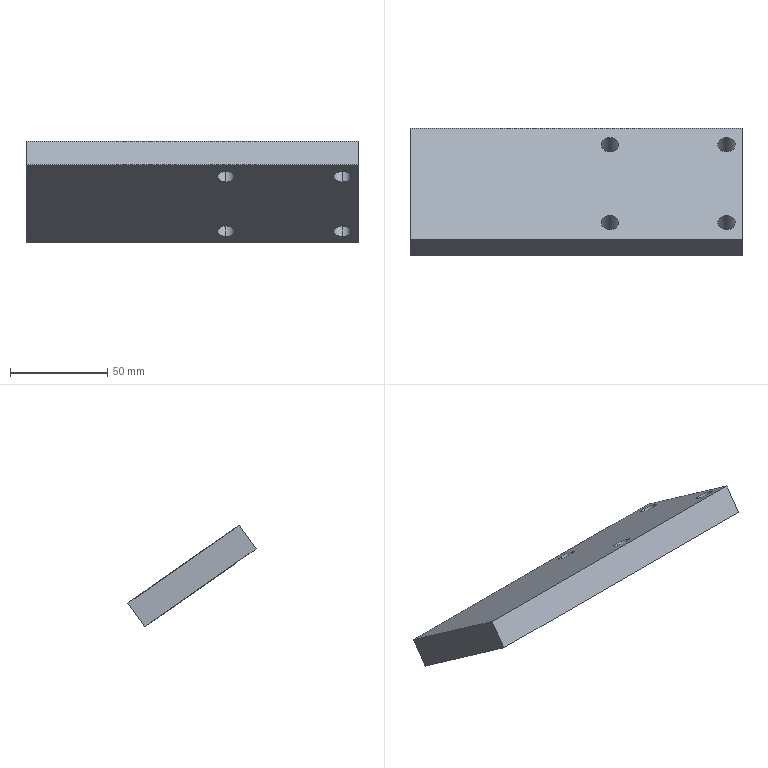Part | STEP file | Positioning_id286_x_t | 1 solid | 14 faces | box 171 x 65.944 x 52.438 mm | volume 175733 mm3 | cylinder 8 | plane 6 | commonest cylinder face diameters 9 x8